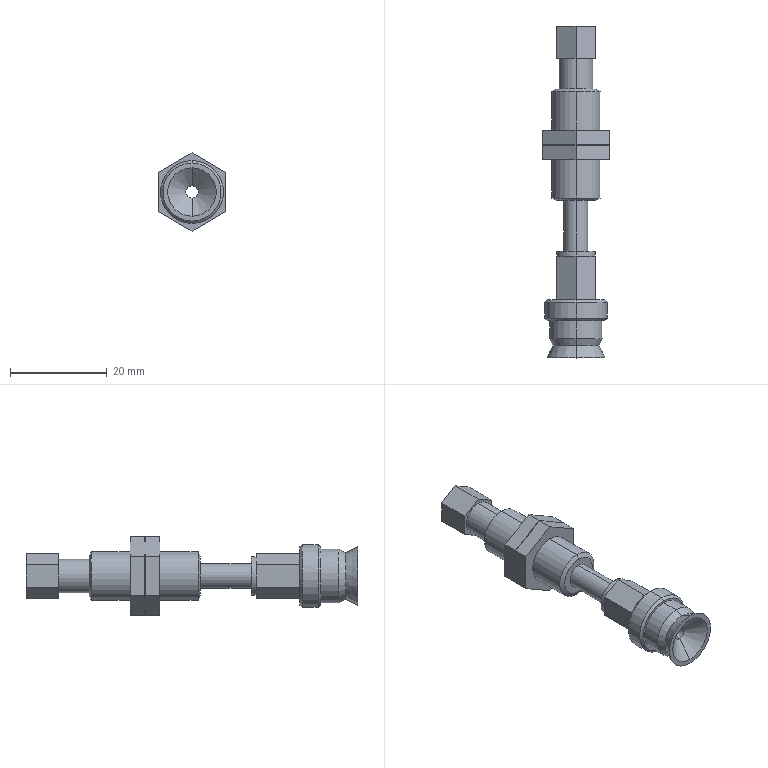Part | STEP file | ZPT10UNJ10_B5_A10_N_ZPT10UNJ10-B5-A10 | 1 solid | 79 faces | box 14 x 68.5 x 16.166 mm | volume 4501 mm3 | plane 43 | cylinder 20 | cone 16 | commonest cylinder face diameters 10 x6 2.5 x2 4.13 x2 5 x2 7 x2 8 x2